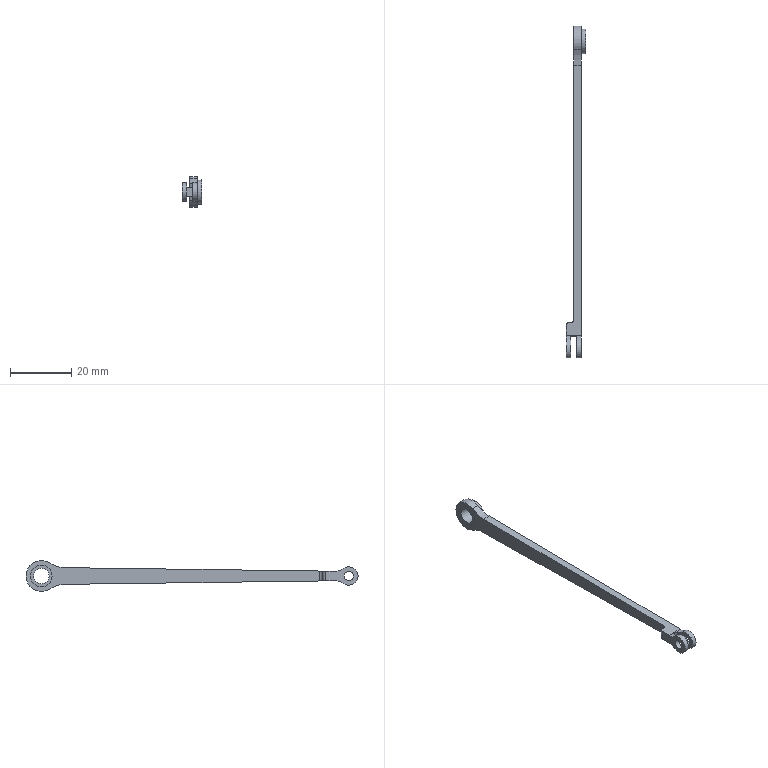Part | STEP file | 2-13 | 2 solids | 27 faces | box 6.5 x 108 x 10 mm | volume 1291 mm3 | cylinder 15 | plane 12 | commonest cylinder face diameters 8 x3 2 x2 3 x2 6 x2 7 x2 20 x2